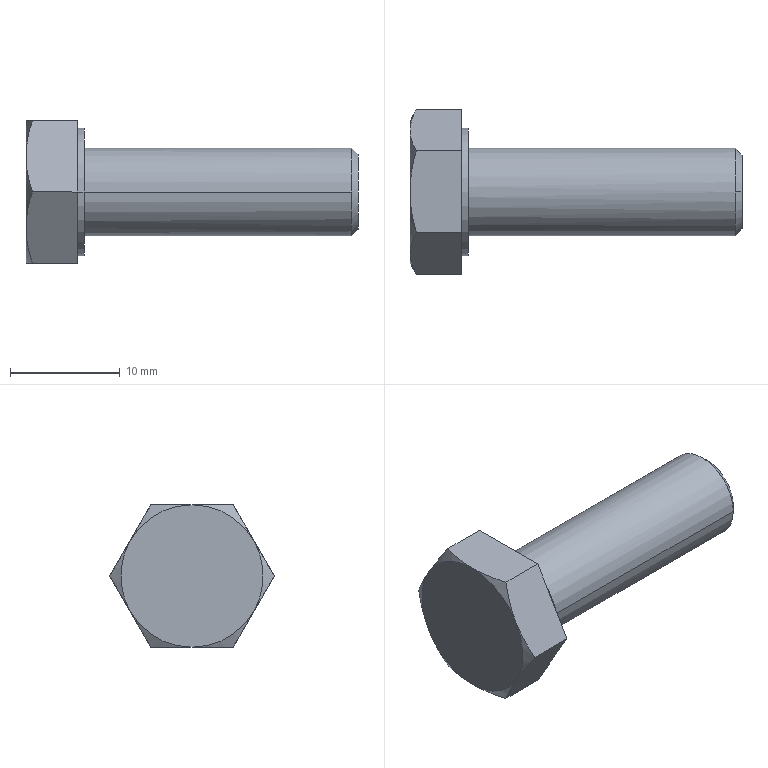Part | STEP file | 1 solid | 22 faces | box 30.3 x 15.011 x 13 mm | volume 2001 mm3 | plane 10 | cone 8 | cylinder 4 | commonest cylinder face diameters 8 x2 11.63 x2